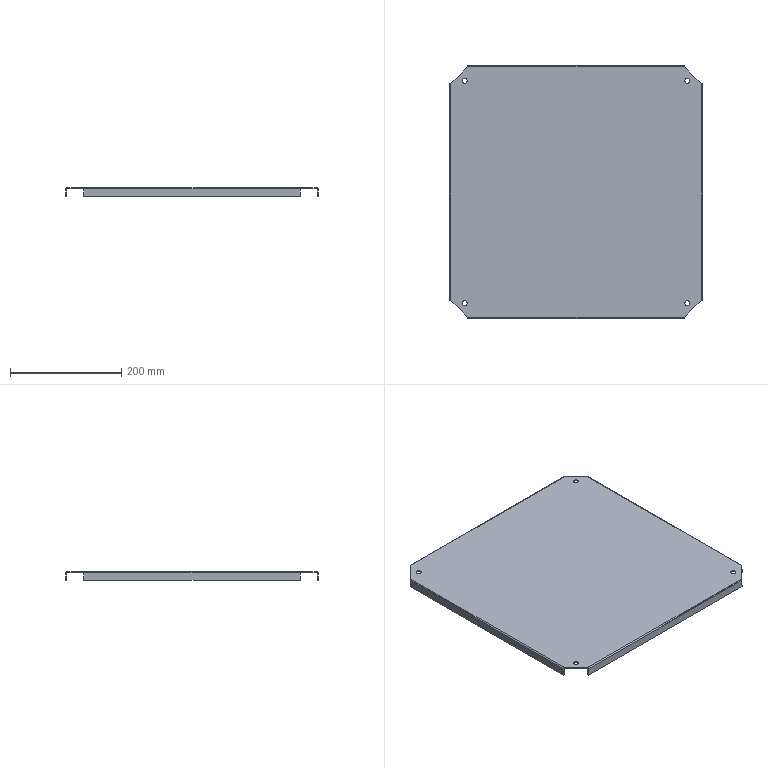Part | SolidWorks | features EdgeFlange 2, LPattern 2, Chamfer 1, FlatPattern 1, ICE 1, SMBaseFlange 1, SheetMetal 1 | 1 solid | 58 faces | box 454 x 454 x 16 mm | volume 449338 mm3 | plane 42 | cylinder 16 | commonest cylinder face diameters 9 x8 0.2 x4 4.2 x4